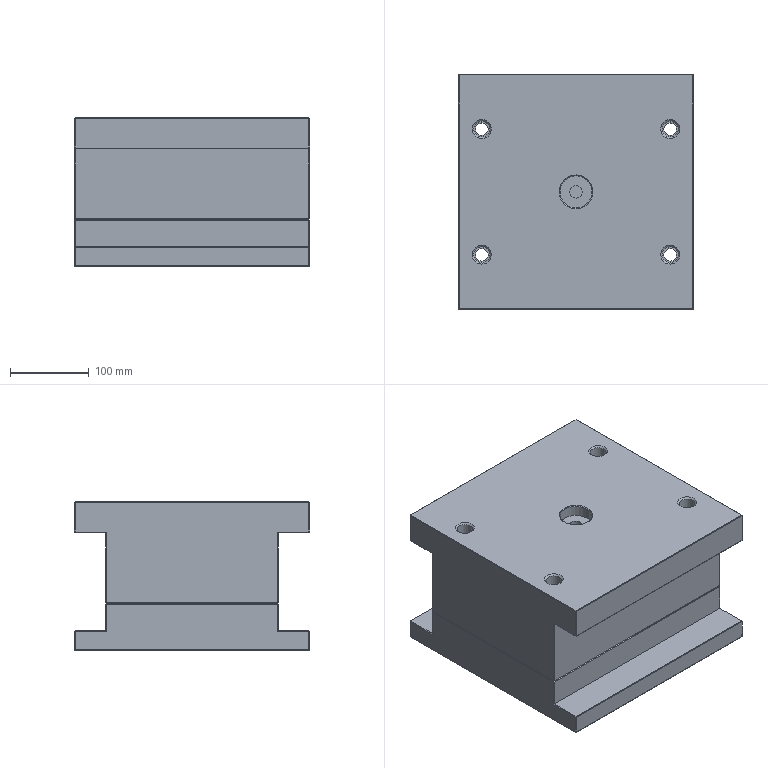NC program | NX | posted with a generic post | part box 300 x 300 x 190 mm
Lines 4668 to 6040 of 6235, first 962 of 1367 lines:
(HOLE_MILLING , TOOL : D10C)
N9334 T10 M6
N9336 G17 G43 G0 G90 X-120. Y80. Z30. S2000 H10 M3
N9338 Z0.5
N9340 G94 G3 X-118.55 Y78.55 R1.45 F1500.
N9342 X-117.1 Y80. R1.45
N9344 X-117.1 Y80. Z0.3 I-2.9 J0.
N9346 X-117.1 Y80. Z0.1 I-2.9 J0.
N9348 X-117.1 Y80. Z-0.1 I-2.9 J0.
N9350 X-117.1 Y80. Z-0.3 I-2.9 J0.
N9352 X-117.1 Y80. Z-0.5 I-2.9 J0.
N9354 X-117.1 Y80. Z-0.7 I-2.9 J0.
N9356 X-117.1 Y80. Z-0.9 I-2.9 J0.
N9358 X-117.1 Y80. Z-1.1 I-2.9 J0.
N9360 X-117.1 Y80. Z-1.3 I-2.9 J0.
N9362 X-117.1 Y80. Z-1.5 I-2.9 J0.
N9364 X-117.1 Y80. Z-1.7 I-2.9 J0.
N9366 X-117.1 Y80. Z-1.9 I-2.9 J0.
N9368 X-117.1 Y80. Z-2.1 I-2.9 J0.
N9370 X-117.1 Y80. Z-2.3 I-2.9 J0.
N9372 X-117.1 Y80. Z-2.5 I-2.9 J0.
N9374 X-117.1 Y80. Z-2.7 I-2.9 J0.
N9376 X-117.1 Y80. Z-2.9 I-2.9 J0.
N9378 X-117.1 Y80. Z-3.1 I-2.9 J0.
N9380 X-117.1 Y80. Z-3.3 I-2.9 J0.
N9382 X-117.1 Y80. Z-3.5 I-2.9 J0.
N9384 X-117.1 Y80. Z-3.7 I-2.9 J0.
N9386 X-117.1 Y80. Z-3.9 I-2.9 J0.
N9388 X-117.1 Y80. Z-4.1 I-2.9 J0.
N9390 X-117.1 Y80. Z-4.3 I-2.9 J0.
N9392 X-117.1 Y80. Z-4.5 I-2.9 J0.
N9394 X-117.1 Y80. Z-4.7 I-2.9 J0.
N9396 X-117.1 Y80. Z-4.9 I-2.9 J0.
N9398 X-117.1 Y80. Z-5.1 I-2.9 J0.
N9400 X-117.1 Y80. Z-5.3 I-2.9 J0.
N9402 X-117.1 Y80. Z-5.5 I-2.9 J0.
N9404 X-117.1 Y80. Z-5.7 I-2.9 J0.
N9406 X-117.1 Y80. Z-5.9 I-2.9 J0.
N9408 X-117.1 Y80. Z-6.1 I-2.9 J0.
N9410 X-117.1 Y80. Z-6.3 I-2.9 J0.
N9412 X-117.1 Y80. Z-6.5 I-2.9 J0.
N9414 X-117.1 Y80. Z-6.7 I-2.9 J0.
N9416 X-117.1 Y80. Z-6.9 I-2.9 J0.
N9418 X-117.1 Y80. Z-7.1 I-2.9 J0.
N9420 X-117.1 Y80. Z-7.3 I-2.9 J0.
N9422 X-117.1 Y80. Z-7.5 I-2.9 J0.
N9424 X-117.1 Y80. Z-7.7 I-2.9 J0.
N9426 X-117.1 Y80. Z-7.9 I-2.9 J0.
N9428 X-117.1 Y80. Z-8.1 I-2.9 J0.
N9430 X-117.1 Y80. Z-8.3 I-2.9 J0.
N9432 X-117.1 Y80. Z-8.5 I-2.9 J0.
N9434 X-117.1 Y80. Z-8.7 I-2.9 J0.
N9436 X-117.1 Y80. Z-8.9 I-2.9 J0.
N9438 X-117.1 Y80. Z-9.1 I-2.9 J0.
N9440 X-117.1 Y80. Z-9.3 I-2.9 J0.
N9442 X-117.1 Y80. Z-9.5 I-2.9 J0.
N9444 X-117.1 Y80. Z-9.7 I-2.9 J0.
N9446 X-117.1 Y80. Z-9.9 I-2.9 J0.
N9448 X-117.1 Y80. Z-10.1 I-2.9 J0.
N9450 X-117.1 Y80. Z-10.3 I-2.9 J0.
N9452 X-117.1 Y80. Z-10.5 I-2.9 J0.
N9454 X-117.1 Y80. Z-10.7 I-2.9 J0.
N9456 X-117.1 Y80. Z-10.9 I-2.9 J0.
N9458 X-117.1 Y80. Z-11.1 I-2.9 J0.
N9460 X-117.1 Y80. Z-11.3 I-2.9 J0.
N9462 X-117.1 Y80. Z-11.5 I-2.9 J0.
N9464 X-117.1 Y80. Z-11.7 I-2.9 J0.
N9466 X-117.1 Y80. Z-11.9 I-2.9 J0.
N9468 X-117.1 Y80. Z-12.1 I-2.9 J0.
N9470 X-117.1 Y80. Z-12.3 I-2.9 J0.
N9472 X-117.1 Y80. Z-12.5 I-2.9 J0.
N9474 X-117.1 Y80. Z-12.7 I-2.9 J0.
N9476 X-117.1 Y80. Z-12.9 I-2.9 J0.
N9478 X-117.1 Y80. Z-13.1 I-2.9 J0.
N9480 X-117.1 Y80. Z-13.3 I-2.9 J0.
N9482 X-117.1 Y80. Z-13.5 I-2.9 J0.
N9484 X-117.1 Y80. Z-13.7 I-2.9 J0.
N9486 X-117.1 Y80. Z-13.9 I-2.9 J0.
N9488 X-117.1 Y80. Z-14.1 I-2.9 J0.
N9490 X-117.1 Y80. Z-14.3 I-2.9 J0.
N9492 X-117.1 Y80. Z-14.5 I-2.9 J0.
N9494 X-117.1 Y80. Z-14.7 I-2.9 J0.
N9496 X-117.1 Y80. Z-14.9 I-2.9 J0.
N9498 X-117.1 Y80. Z-15.1 I-2.9 J0.
N9500 X-117.1 Y80. Z-15.3 I-2.9 J0.
N9502 X-117.1 Y80. Z-15.5 I-2.9 J0.
N9504 X-117.1 Y80. Z-15.7 I-2.9 J0.
N9506 X-117.1 Y80. Z-15.9 I-2.9 J0.
N9508 X-117.1 Y80. Z-16.1 I-2.9 J0.
N9510 X-117.1 Y80. Z-16.3 I-2.9 J0.
N9512 X-117.1 Y80. Z-16.5 I-2.9 J0.
N9514 X-117.1 Y80. Z-16.7 I-2.9 J0.
N9516 X-117.1 Y80. Z-16.9 I-2.9 J0.
N9518 X-117.1 Y80. Z-17.1 I-2.9 J0.
N9520 X-117.1 Y80. Z-17.3 I-2.9 J0.
N9522 X-117.1 Y80. Z-17.5 I-2.9 J0.
N9524 X-117.1 Y80. Z-17.7 I-2.9 J0.
N9526 X-117.1 Y80. Z-17.9 I-2.9 J0.
N9528 X-117.1 Y80. Z-18.1 I-2.9 J0.
N9530 X-117.1 Y80. Z-18.3 I-2.9 J0.
N9532 X-117.1 Y80. Z-18.5 I-2.9 J0.
N9534 X-117.1 Y80. Z-18.7 I-2.9 J0.
N9536 X-117.1 Y80. Z-18.9 I-2.9 J0.
N9538 X-117.1 Y80. Z-19.1 I-2.9 J0.
N9540 X-117.1 Y80. Z-19.3 I-2.9 J0.
N9542 X-117.1 Y80. Z-19.5 I-2.9 J0.
N9544 X-117.1 Y80. Z-19.7 I-2.9 J0.
N9546 X-117.1 Y80. Z-19.9 I-2.9 J0.
N9548 X-117.1 Y80. Z-20.1 I-2.9 J0.
N9550 X-117.1 Y80. Z-20.3 I-2.9 J0.
N9552 X-117.1 Y80. Z-20.5 I-2.9 J0.
N9554 X-117.1 Y80. Z-20.7 I-2.9 J0.
N9556 X-117.1 Y80. Z-20.9 I-2.9 J0.
N9558 X-117.1 Y80. Z-21.1 I-2.9 J0.
N9560 X-117.1 Y80. Z-21.3 I-2.9 J0.
N9562 X-117.1 Y80. Z-21.5 I-2.9 J0.
N9564 X-117.1 Y80. Z-21.7 I-2.9 J0.
N9566 X-117.1 Y80. Z-21.9 I-2.9 J0.
N9568 X-117.1 Y80. Z-22.1 I-2.9 J0.
N9570 X-117.1 Y80. Z-22.3 I-2.9 J0.
N9572 X-117.1 Y80. Z-22.5 I-2.9 J0.
N9574 X-117.1 Y80. Z-22.7 I-2.9 J0.
N9576 X-117.1 Y80. Z-22.9 I-2.9 J0.
N9578 X-117.1 Y80. Z-23.1 I-2.9 J0.
N9580 X-117.1 Y80. Z-23.3 I-2.9 J0.
N9582 X-117.1 Y80. Z-23.5 I-2.9 J0.
N9584 X-117.1 Y80. Z-23.7 I-2.9 J0.
N9586 X-117.1 Y80. Z-23.9 I-2.9 J0.
N9588 X-117.1 Y80. Z-24.1 I-2.9 J0.
N9590 X-117.1 Y80. Z-24.3 I-2.9 J0.
N9592 X-117.1 Y80. Z-24.5 I-2.9 J0.
N9594 X-117.1 Y80. Z-24.7 I-2.9 J0.
N9596 X-117.1 Y80. Z-24.9 I-2.9 J0.
N9598 X-117.1 Y80. Z-25.1 I-2.9 J0.
N9600 X-117.1 Y80. Z-25.3 I-2.9 J0.
N9602 X-117.1 Y80. Z-25.5 I-2.9 J0.
N9604 X-117.1 Y80. Z-25.7 I-2.9 J0.
N9606 X-117.1 Y80. Z-25.9 I-2.9 J0.
N9608 X-117.1 Y80. Z-26.1 I-2.9 J0.
N9610 X-117.1 Y80. Z-26.3 I-2.9 J0.
N9612 X-117.1 Y80. Z-26.5 I-2.9 J0.
N9614 X-117.1 Y80. Z-26.7 I-2.9 J0.
N9616 X-117.1 Y80. Z-26.9 I-2.9 J0.
N9618 X-117.1 Y80. Z-27.1 I-2.9 J0.
N9620 X-117.1 Y80. Z-27.3 I-2.9 J0.
N9622 X-117.1 Y80. Z-27.5 I-2.9 J0.
N9624 X-117.1 Y80. Z-27.7 I-2.9 J0.
N9626 X-117.1 Y80. Z-27.9 I-2.9 J0.
N9628 X-117.1 Y80. Z-28.1 I-2.9 J0.
N9630 X-117.1 Y80. Z-28.3 I-2.9 J0.
N9632 X-117.1 Y80. Z-28.5 I-2.9 J0.
N9634 X-117.1 Y80. Z-28.7 I-2.9 J0.
N9636 X-117.1 Y80. Z-28.9 I-2.9 J0.
N9638 X-117.1 Y80. Z-29.1 I-2.9 J0.
N9640 X-117.1 Y80. Z-29.3 I-2.9 J0.
N9642 X-117.1 Y80. Z-29.5 I-2.9 J0.
N9644 X-117.1 Y80. Z-29.7 I-2.9 J0.
N9646 X-117.1 Y80. Z-29.9 I-2.9 J0.
N9648 X-117.1 Y80. Z-30.1 I-2.9 J0.
N9650 X-117.1 Y80. Z-30.3 I-2.9 J0.
N9652 X-117.1 Y80. Z-30.5 I-2.9 J0.
N9654 X-117.1 Y80. Z-30.7 I-2.9 J0.
N9656 X-117.1 Y80. Z-30.9 I-2.9 J0.
N9658 X-117.1 Y80. Z-31.1 I-2.9 J0.
N9660 X-117.1 Y80. Z-31.3 I-2.9 J0.
N9662 X-117.1 Y80. Z-31.5 I-2.9 J0.
N9664 X-117.1 Y80. Z-31.7 I-2.9 J0.
N9666 X-117.1 Y80. Z-31.9 I-2.9 J0.
N9668 X-117.1 Y80. Z-32.1 I-2.9 J0.
N9670 X-117.1 Y80. Z-32.3 I-2.9 J0.
N9672 X-117.1 Y80. Z-32.5 I-2.9 J0.
N9674 X-117.1 Y80. Z-32.7 I-2.9 J0.
N9676 X-117.1 Y80. Z-32.9 I-2.9 J0.
N9678 X-117.1 Y80. Z-33.1 I-2.9 J0.
N9680 X-117.1 Y80. Z-33.3 I-2.9 J0.
N9682 X-117.1 Y80. Z-33.5 I-2.9 J0.
N9684 X-117.1 Y80. Z-33.7 I-2.9 J0.
N9686 X-117.1 Y80. Z-33.9 I-2.9 J0.
N9688 X-117.1 Y80. Z-34.1 I-2.9 J0.
N9690 X-117.1 Y80. Z-34.3 I-2.9 J0.
N9692 X-117.1 Y80. Z-34.5 I-2.9 J0.
N9694 X-117.1 Y80. Z-34.7 I-2.9 J0.
N9696 X-117.1 Y80. Z-34.9 I-2.9 J0.
N9698 X-117.1 Y80. Z-35.1 I-2.9 J0.
N9700 X-117.1 Y80. Z-35.3 I-2.9 J0.
N9702 X-117.1 Y80. Z-35.5 I-2.9 J0.
N9704 X-117.1 Y80. Z-35.7 I-2.9 J0.
N9706 X-117.1 Y80. Z-35.9 I-2.9 J0.
N9708 X-117.1 Y80. Z-36.1 I-2.9 J0.
N9710 X-117.1 Y80. Z-36.3 I-2.9 J0.
N9712 X-117.1 Y80. Z-36.5 I-2.9 J0.
N9714 X-117.1 Y80. Z-36.7 I-2.9 J0.
N9716 X-117.1 Y80. Z-36.9 I-2.9 J0.
N9718 X-117.1 Y80. Z-37.1 I-2.9 J0.
N9720 X-117.1 Y80. Z-37.3 I-2.9 J0.
N9722 X-117.1 Y80. Z-37.5 I-2.9 J0.
N9724 X-117.1 Y80. Z-37.7 I-2.9 J0.
N9726 X-117.1 Y80. Z-37.9 I-2.9 J0.
N9728 X-117.1 Y80. Z-38.1 I-2.9 J0.
N9730 X-117.1 Y80. Z-38.3 I-2.9 J0.
N9732 X-117.1 Y80. Z-38.5 I-2.9 J0.
N9734 X-117.1 Y80. Z-38.7 I-2.9 J0.
N9736 X-117.1 Y80. Z-38.9 I-2.9 J0.
N9738 X-117.1 Y80. Z-39.1 I-2.9 J0.
N9740 X-117.1 Y80. Z-39.3 I-2.9 J0.
N9742 X-117.1 Y80. Z-39.5 I-2.9 J0.
N9744 X-117.1 Y80. Z-39.7 I-2.9 J0.
N9746 X-117.1 Y80. Z-39.9 I-2.9 J0.
N9748 X-117.1 Y80. Z-40.1 I-2.9 J0.
N9750 X-117.1 Y80. Z-40.3 I-2.9 J0.
N9752 X-117.1 Y80. Z-40.5 I-2.9 J0.
N9754 X-117.1 Y80. Z-40.7 I-2.9 J0.
N9756 X-117.1 Y80. Z-40.9 I-2.9 J0.
N9758 X-117.1 Y80. Z-41.1 I-2.9 J0.
N9760 X-117.1 Y80. Z-41.3 I-2.9 J0.
N9762 X-117.1 Y80. Z-41.5 I-2.9 J0.
N9764 X-117.1 Y80. Z-41.7 I-2.9 J0.
N9766 X-117.1 Y80. Z-41.9 I-2.9 J0.
N9768 X-117.1 Y80. Z-42.1 I-2.9 J0.
N9770 X-117.1 Y80. Z-42.3 I-2.9 J0.
N9772 X-117.1 Y80. Z-42.5 I-2.9 J0.
N9774 X-117.1 Y80. Z-42.7 I-2.9 J0.
N9776 X-117.1 Y80. Z-42.9 I-2.9 J0.
N9778 X-117.1 Y80. Z-43.1 I-2.9 J0.
N9780 X-117.1 Y80. Z-43.3 I-2.9 J0.
N9782 X-117.1 Y80. Z-43.5 I-2.9 J0.
N9784 X-117.1 Y80. Z-43.7 I-2.9 J0.
N9786 X-117.1 Y80. Z-43.9 I-2.9 J0.
N9788 X-117.1 Y80. Z-44.1 I-2.9 J0.
N9790 X-117.1 Y80. Z-44.3 I-2.9 J0.
N9792 X-117.1 Y80. Z-44.5 I-2.9 J0.
N9794 X-117.1 Y80. Z-44.7 I-2.9 J0.
N9796 X-117.1 Y80. Z-44.9 I-2.9 J0.
N9798 X-117.1 Y80. Z-45.1 I-2.9 J0.
N9800 X-117.1 Y80. Z-45.3 I-2.9 J0.
N9802 X-117.1 Y80. Z-45.5 I-2.9 J0.
N9804 X-117.1 Y80. Z-45.7 I-2.9 J0.
N9806 X-117.1 Y80. Z-45.9 I-2.9 J0.
N9808 X-117.1 Y80. Z-46.1 I-2.9 J0.
N9810 X-117.1 Y80. Z-46.3 I-2.9 J0.
N9812 X-117.1 Y80. Z-46.5 I-2.9 J0.
N9814 X-117.1 Y80. Z-46.7 I-2.9 J0.
N9816 X-117.1 Y80. Z-46.9 I-2.9 J0.
N9818 X-117.1 Y80. Z-47.1 I-2.9 J0.
N9820 X-117.1 Y80. Z-47.3 I-2.9 J0.
N9822 X-117.1 Y80. Z-47.5 I-2.9 J0.
N9824 X-117.1 Y80. Z-47.7 I-2.9 J0.
N9826 X-117.1 Y80. Z-47.9 I-2.9 J0.
N9828 X-117.1 Y80. Z-48.1 I-2.9 J0.
N9830 X-117.1 Y80. Z-48.3 I-2.9 J0.
N9832 X-117.1 Y80. Z-48.5 I-2.9 J0.
N9834 X-117.1 Y80. Z-48.7 I-2.9 J0.
N9836 X-117.1 Y80. Z-48.9 I-2.9 J0.
N9838 X-117.1 Y80. Z-49.1 I-2.9 J0.
N9840 X-117.1 Y80. Z-49.3 I-2.9 J0.
N9842 X-117.1 Y80. Z-49.5 I-2.9 J0.
N9844 X-117.1 Y80. Z-49.7 I-2.9 J0.
N9846 X-117.1 Y80. Z-49.9 I-2.9 J0.
N9848 X-117.1 Y80. Z-50.1 I-2.9 J0.
N9850 X-117.1 Y80. Z-50.3 I-2.9 J0.
N9852 X-117.1 Y80. Z-50.5 I-2.9 J0.
N9854 X-117.1 Y80. Z-50.7 I-2.9 J0.
N9856 X-117.1 Y80. Z-50.9 I-2.9 J0.
N9858 X-117.1 Y80. Z-51.1 I-2.9 J0.
N9860 X-117.1 Y80. Z-51.3 I-2.9 J0.
N9862 X-117.1 Y80. Z-51.5 I-2.9 J0.
N9864 X-117.1 Y80. Z-51.7 I-2.9 J0.
N9866 X-117.1 Y80. Z-51.9 I-2.9 J0.
N9868 X-117.1 Y80. Z-52.1 I-2.9 J0.
N9870 X-117.1 Y80. Z-52.3 I-2.9 J0.
N9872 X-117.1 Y80. Z-52.5 I-2.9 J0.
N9874 X-117.1 Y80. Z-52.7 I-2.9 J0.
N9876 X-117.1 Y80. Z-52.9 I-2.9 J0.
N9878 X-117.1 Y80. Z-53.1 I-2.9 J0.
N9880 X-117.1 Y80. Z-53.3 I-2.9 J0.
N9882 X-117.1 Y80. Z-53.5 I-2.9 J0.
N9884 X-117.1 Y80. Z-53.7 I-2.9 J0.
N9886 X-117.1 Y80. Z-53.9 I-2.9 J0.
N9888 X-117.1 Y80. Z-54.1 I-2.9 J0.
N9890 X-117.1 Y80. Z-54.3 I-2.9 J0.
N9892 X-117.1 Y80. Z-54.5 I-2.9 J0.
N9894 X-117.1 Y80. Z-54.7 I-2.9 J0.
N9896 X-117.1 Y80. Z-54.9 I-2.9 J0.
N9898 X-117.1 Y80. Z-55.1 I-2.9 J0.
N9900 X-117.1 Y80. Z-55.3 I-2.9 J0.
N9902 X-117.1 Y80. Z-55.5 I-2.9 J0.
N9904 X-117.1 Y80. Z-55.7 I-2.9 J0.
N9906 X-117.1 Y80. Z-55.9 I-2.9 J0.
N9908 X-117.1 Y80. Z-56.1 I-2.9 J0.
N9910 X-117.1 Y80. Z-56.3 I-2.9 J0.
N9912 X-117.1 Y80. Z-56.5 I-2.9 J0.
N9914 X-117.1 Y80. Z-56.7 I-2.9 J0.
N9916 X-117.1 Y80. Z-56.9 I-2.9 J0.
N9918 X-117.1 Y80. Z-57.1 I-2.9 J0.
N9920 X-117.1 Y80. Z-57.3 I-2.9 J0.
N9922 X-117.1 Y80. Z-57.5 I-2.9 J0.
N9924 X-117.1 Y80. Z-57.7 I-2.9 J0.
N9926 X-117.1 Y80. Z-57.9 I-2.9 J0.
N9928 X-117.1 Y80. Z-58.1 I-2.9 J0.
N9930 X-117.1 Y80. Z-58.3 I-2.9 J0.
N9932 X-117.1 Y80. Z-58.5 I-2.9 J0.
N9934 X-117.1 Y80. Z-58.7 I-2.9 J0.
N9936 X-117.1 Y80. Z-58.9 I-2.9 J0.
N9938 X-117.1 Y80. Z-59.1 I-2.9 J0.
N9940 X-117.1 Y80. Z-59.3 I-2.9 J0.
N9942 X-117.1 Y80. Z-59.5 I-2.9 J0.
N9944 X-117.1 Y80. Z-59.7 I-2.9 J0.
N9946 X-117.1 Y80. Z-59.9 I-2.9 J0.
N9948 X-122.9 Y80. Z-60. I-2.9 J0.
N9950 X-120. Y77.1 R2.9
N9952 X-122.9 Y80. R-2.9
N9954 X-121.45 Y78.55 R1.45
N9956 X-120. Y80. R1.45
N9958 G0 Z30.
N9960 Y-80.
N9962 Z0.5
N9964 G3 X-118.55 Y-81.45 R1.45
N9966 X-117.1 Y-80. R1.45
N9968 X-117.1 Y-80. Z0.3 I-2.9 J0.
N9970 X-117.1 Y-80. Z0.1 I-2.9 J0.
N9972 X-117.1 Y-80. Z-0.1 I-2.9 J0.
N9974 X-117.1 Y-80. Z-0.3 I-2.9 J0.
N9976 X-117.1 Y-80. Z-0.5 I-2.9 J0.
N9978 X-117.1 Y-80. Z-0.7 I-2.9 J0.
N9980 X-117.1 Y-80. Z-0.9 I-2.9 J0.
N9982 X-117.1 Y-80. Z-1.1 I-2.9 J0.
N9984 X-117.1 Y-80. Z-1.3 I-2.9 J0.
N9986 X-117.1 Y-80. Z-1.5 I-2.9 J0.
N9988 X-117.1 Y-80. Z-1.7 I-2.9 J0.
N9990 X-117.1 Y-80. Z-1.9 I-2.9 J0.
N9992 X-117.1 Y-80. Z-2.1 I-2.9 J0.
N9994 X-117.1 Y-80. Z-2.3 I-2.9 J0.
N9996 X-117.1 Y-80. Z-2.5 I-2.9 J0.
N9998 X-117.1 Y-80. Z-2.7 I-2.9 J0.
N10000 X-117.1 Y-80. Z-2.9 I-2.9 J0.
N10002 X-117.1 Y-80. Z-3.1 I-2.9 J0.
N10004 X-117.1 Y-80. Z-3.3 I-2.9 J0.
N10006 X-117.1 Y-80. Z-3.5 I-2.9 J0.
N10008 X-117.1 Y-80. Z-3.7 I-2.9 J0.
N10010 X-117.1 Y-80. Z-3.9 I-2.9 J0.
N10012 X-117.1 Y-80. Z-4.1 I-2.9 J0.
N10014 X-117.1 Y-80. Z-4.3 I-2.9 J0.
N10016 X-117.1 Y-80. Z-4.5 I-2.9 J0.
N10018 X-117.1 Y-80. Z-4.7 I-2.9 J0.
N10020 X-117.1 Y-80. Z-4.9 I-2.9 J0.
N10022 X-117.1 Y-80. Z-5.1 I-2.9 J0.
N10024 X-117.1 Y-80. Z-5.3 I-2.9 J0.
N10026 X-117.1 Y-80. Z-5.5 I-2.9 J0.
N10028 X-117.1 Y-80. Z-5.7 I-2.9 J0.
N10030 X-117.1 Y-80. Z-5.9 I-2.9 J0.
N10032 X-117.1 Y-80. Z-6.1 I-2.9 J0.
N10034 X-117.1 Y-80. Z-6.3 I-2.9 J0.
N10036 X-117.1 Y-80. Z-6.5 I-2.9 J0.
N10038 X-117.1 Y-80. Z-6.7 I-2.9 J0.
N10040 X-117.1 Y-80. Z-6.9 I-2.9 J0.
N10042 X-117.1 Y-80. Z-7.1 I-2.9 J0.
N10044 X-117.1 Y-80. Z-7.3 I-2.9 J0.
N10046 X-117.1 Y-80. Z-7.5 I-2.9 J0.
N10048 X-117.1 Y-80. Z-7.7 I-2.9 J0.
N10050 X-117.1 Y-80. Z-7.9 I-2.9 J0.
N10052 X-117.1 Y-80. Z-8.1 I-2.9 J0.
N10054 X-117.1 Y-80. Z-8.3 I-2.9 J0.
N10056 X-117.1 Y-80. Z-8.5 I-2.9 J0.
N10058 X-117.1 Y-80. Z-8.7 I-2.9 J0.
N10060 X-117.1 Y-80. Z-8.9 I-2.9 J0.
N10062 X-117.1 Y-80. Z-9.1 I-2.9 J0.
N10064 X-117.1 Y-80. Z-9.3 I-2.9 J0.
N10066 X-117.1 Y-80. Z-9.5 I-2.9 J0.
N10068 X-117.1 Y-80. Z-9.7 I-2.9 J0.
N10070 X-117.1 Y-80. Z-9.9 I-2.9 J0.
N10072 X-117.1 Y-80. Z-10.1 I-2.9 J0.
N10074 X-117.1 Y-80. Z-10.3 I-2.9 J0.
N10076 X-117.1 Y-80. Z-10.5 I-2.9 J0.
N10078 X-117.1 Y-80. Z-10.7 I-2.9 J0.
N10080 X-117.1 Y-80. Z-10.9 I-2.9 J0.
N10082 X-117.1 Y-80. Z-11.1 I-2.9 J0.
N10084 X-117.1 Y-80. Z-11.3 I-2.9 J0.
N10086 X-117.1 Y-80. Z-11.5 I-2.9 J0.
N10088 X-117.1 Y-80. Z-11.7 I-2.9 J0.
N10090 X-117.1 Y-80. Z-11.9 I-2.9 J0.
N10092 X-117.1 Y-80. Z-12.1 I-2.9 J0.
N10094 X-117.1 Y-80. Z-12.3 I-2.9 J0.
N10096 X-117.1 Y-80. Z-12.5 I-2.9 J0.
N10098 X-117.1 Y-80. Z-12.7 I-2.9 J0.
N10100 X-117.1 Y-80. Z-12.9 I-2.9 J0.
N10102 X-117.1 Y-80. Z-13.1 I-2.9 J0.
N10104 X-117.1 Y-80. Z-13.3 I-2.9 J0.
N10106 X-117.1 Y-80. Z-13.5 I-2.9 J0.
N10108 X-117.1 Y-80. Z-13.7 I-2.9 J0.
N10110 X-117.1 Y-80. Z-13.9 I-2.9 J0.
N10112 X-117.1 Y-80. Z-14.1 I-2.9 J0.
N10114 X-117.1 Y-80. Z-14.3 I-2.9 J0.
N10116 X-117.1 Y-80. Z-14.5 I-2.9 J0.
N10118 X-117.1 Y-80. Z-14.7 I-2.9 J0.
N10120 X-117.1 Y-80. Z-14.9 I-2.9 J0.
N10122 X-117.1 Y-80. Z-15.1 I-2.9 J0.
N10124 X-117.1 Y-80. Z-15.3 I-2.9 J0.
N10126 X-117.1 Y-80. Z-15.5 I-2.9 J0.
N10128 X-117.1 Y-80. Z-15.7 I-2.9 J0.
N10130 X-117.1 Y-80. Z-15.9 I-2.9 J0.
N10132 X-117.1 Y-80. Z-16.1 I-2.9 J0.
N10134 X-117.1 Y-80. Z-16.3 I-2.9 J0.
N10136 X-117.1 Y-80. Z-16.5 I-2.9 J0.
N10138 X-117.1 Y-80. Z-16.7 I-2.9 J0.
N10140 X-117.1 Y-80. Z-16.9 I-2.9 J0.
N10142 X-117.1 Y-80. Z-17.1 I-2.9 J0.
N10144 X-117.1 Y-80. Z-17.3 I-2.9 J0.
N10146 X-117.1 Y-80. Z-17.5 I-2.9 J0.
N10148 X-117.1 Y-80. Z-17.7 I-2.9 J0.
N10150 X-117.1 Y-80. Z-17.9 I-2.9 J0.
N10152 X-117.1 Y-80. Z-18.1 I-2.9 J0.
N10154 X-117.1 Y-80. Z-18.3 I-2.9 J0.
N10156 X-117.1 Y-80. Z-18.5 I-2.9 J0.
N10158 X-117.1 Y-80. Z-18.7 I-2.9 J0.
N10160 X-117.1 Y-80. Z-18.9 I-2.9 J0.
N10162 X-117.1 Y-80. Z-19.1 I-2.9 J0.
N10164 X-117.1 Y-80. Z-19.3 I-2.9 J0.
N10166 X-117.1 Y-80. Z-19.5 I-2.9 J0.
N10168 X-117.1 Y-80. Z-19.7 I-2.9 J0.
N10170 X-117.1 Y-80. Z-19.9 I-2.9 J0.
N10172 X-117.1 Y-80. Z-20.1 I-2.9 J0.
N10174 X-117.1 Y-80. Z-20.3 I-2.9 J0.
N10176 X-117.1 Y-80. Z-20.5 I-2.9 J0.
N10178 X-117.1 Y-80. Z-20.7 I-2.9 J0.
N10180 X-117.1 Y-80. Z-20.9 I-2.9 J0.
N10182 X-117.1 Y-80. Z-21.1 I-2.9 J0.
N10184 X-117.1 Y-80. Z-21.3 I-2.9 J0.
N10186 X-117.1 Y-80. Z-21.5 I-2.9 J0.
N10188 X-117.1 Y-80. Z-21.7 I-2.9 J0.
N10190 X-117.1 Y-80. Z-21.9 I-2.9 J0.
N10192 X-117.1 Y-80. Z-22.1 I-2.9 J0.
N10194 X-117.1 Y-80. Z-22.3 I-2.9 J0.
N10196 X-117.1 Y-80. Z-22.5 I-2.9 J0.
N10198 X-117.1 Y-80. Z-22.7 I-2.9 J0.
N10200 X-117.1 Y-80. Z-22.9 I-2.9 J0.
N10202 X-117.1 Y-80. Z-23.1 I-2.9 J0.
N10204 X-117.1 Y-80. Z-23.3 I-2.9 J0.
N10206 X-117.1 Y-80. Z-23.5 I-2.9 J0.
N10208 X-117.1 Y-80. Z-23.7 I-2.9 J0.
N10210 X-117.1 Y-80. Z-23.9 I-2.9 J0.
N10212 X-117.1 Y-80. Z-24.1 I-2.9 J0.
N10214 X-117.1 Y-80. Z-24.3 I-2.9 J0.
N10216 X-117.1 Y-80. Z-24.5 I-2.9 J0.
N10218 X-117.1 Y-80. Z-24.7 I-2.9 J0.
N10220 X-117.1 Y-80. Z-24.9 I-2.9 J0.
N10222 X-117.1 Y-80. Z-25.1 I-2.9 J0.
N10224 X-117.1 Y-80. Z-25.3 I-2.9 J0.
N10226 X-117.1 Y-80. Z-25.5 I-2.9 J0.
N10228 X-117.1 Y-80. Z-25.7 I-2.9 J0.
N10230 X-117.1 Y-80. Z-25.9 I-2.9 J0.
N10232 X-117.1 Y-80. Z-26.1 I-2.9 J0.
N10234 X-117.1 Y-80. Z-26.3 I-2.9 J0.
N10236 X-117.1 Y-80. Z-26.5 I-2.9 J0.
N10238 X-117.1 Y-80. Z-26.7 I-2.9 J0.
N10240 X-117.1 Y-80. Z-26.9 I-2.9 J0.
N10242 X-117.1 Y-80. Z-27.1 I-2.9 J0.
N10244 X-117.1 Y-80. Z-27.3 I-2.9 J0.
N10246 X-117.1 Y-80. Z-27.5 I-2.9 J0.
N10248 X-117.1 Y-80. Z-27.7 I-2.9 J0.
N10250 X-117.1 Y-80. Z-27.9 I-2.9 J0.
N10252 X-117.1 Y-80. Z-28.1 I-2.9 J0.
N10254 X-117.1 Y-80. Z-28.3 I-2.9 J0.
N10256 X-117.1 Y-80. Z-28.5 I-2.9 J0.
N10258 X-117.1 Y-80. Z-28.7 I-2.9 J0.
N10260 X-117.1 Y-80. Z-28.9 I-2.9 J0.
N10262 X-117.1 Y-80. Z-29.1 I-2.9 J0.
N10264 X-117.1 Y-80. Z-29.3 I-2.9 J0.
N10266 X-117.1 Y-80. Z-29.5 I-2.9 J0.
N10268 X-117.1 Y-80. Z-29.7 I-2.9 J0.
N10270 X-117.1 Y-80. Z-29.9 I-2.9 J0.
N10272 X-117.1 Y-80. Z-30.1 I-2.9 J0.
N10274 X-117.1 Y-80. Z-30.3 I-2.9 J0.
N10276 X-117.1 Y-80. Z-30.5 I-2.9 J0.
N10278 X-117.1 Y-80. Z-30.7 I-2.9 J0.
N10280 X-117.1 Y-80. Z-30.9 I-2.9 J0.
N10282 X-117.1 Y-80. Z-31.1 I-2.9 J0.
N10284 X-117.1 Y-80. Z-31.3 I-2.9 J0.
N10286 X-117.1 Y-80. Z-31.5 I-2.9 J0.
N10288 X-117.1 Y-80. Z-31.7 I-2.9 J0.
N10290 X-117.1 Y-80. Z-31.9 I-2.9 J0.
N10292 X-117.1 Y-80. Z-32.1 I-2.9 J0.
N10294 X-117.1 Y-80. Z-32.3 I-2.9 J0.
N10296 X-117.1 Y-80. Z-32.5 I-2.9 J0.
N10298 X-117.1 Y-80. Z-32.7 I-2.9 J0.
N10300 X-117.1 Y-80. Z-32.9 I-2.9 J0.
N10302 X-117.1 Y-80. Z-33.1 I-2.9 J0.
N10304 X-117.1 Y-80. Z-33.3 I-2.9 J0.
N10306 X-117.1 Y-80. Z-33.5 I-2.9 J0.
N10308 X-117.1 Y-80. Z-33.7 I-2.9 J0.
N10310 X-117.1 Y-80. Z-33.9 I-2.9 J0.
N10312 X-117.1 Y-80. Z-34.1 I-2.9 J0.
N10314 X-117.1 Y-80. Z-34.3 I-2.9 J0.
N10316 X-117.1 Y-80. Z-34.5 I-2.9 J0.
N10318 X-117.1 Y-80. Z-34.7 I-2.9 J0.
N10320 X-117.1 Y-80. Z-34.9 I-2.9 J0.
N10322 X-117.1 Y-80. Z-35.1 I-2.9 J0.
N10324 X-117.1 Y-80. Z-35.3 I-2.9 J0.
N10326 X-117.1 Y-80. Z-35.5 I-2.9 J0.
N10328 X-117.1 Y-80. Z-35.7 I-2.9 J0.
N10330 X-117.1 Y-80. Z-35.9 I-2.9 J0.
N10332 X-117.1 Y-80. Z-36.1 I-2.9 J0.
N10334 X-117.1 Y-80. Z-36.3 I-2.9 J0.
N10336 X-117.1 Y-80. Z-36.5 I-2.9 J0.
N10338 X-117.1 Y-80. Z-36.7 I-2.9 J0.
N10340 X-117.1 Y-80. Z-36.9 I-2.9 J0.
N10342 X-117.1 Y-80. Z-37.1 I-2.9 J0.
N10344 X-117.1 Y-80. Z-37.3 I-2.9 J0.
N10346 X-117.1 Y-80. Z-37.5 I-2.9 J0.
N10348 X-117.1 Y-80. Z-37.7 I-2.9 J0.
N10350 X-117.1 Y-80. Z-37.9 I-2.9 J0.
N10352 X-117.1 Y-80. Z-38.1 I-2.9 J0.
N10354 X-117.1 Y-80. Z-38.3 I-2.9 J0.
N10356 X-117.1 Y-80. Z-38.5 I-2.9 J0.
N10358 X-117.1 Y-80. Z-38.7 I-2.9 J0.
N10360 X-117.1 Y-80. Z-38.9 I-2.9 J0.
N10362 X-117.1 Y-80. Z-39.1 I-2.9 J0.
N10364 X-117.1 Y-80. Z-39.3 I-2.9 J0.
N10366 X-117.1 Y-80. Z-39.5 I-2.9 J0.
N10368 X-117.1 Y-80. Z-39.7 I-2.9 J0.
N10370 X-117.1 Y-80. Z-39.9 I-2.9 J0.
N10372 X-117.1 Y-80. Z-40.1 I-2.9 J0.
N10374 X-117.1 Y-80. Z-40.3 I-2.9 J0.
N10376 X-117.1 Y-80. Z-40.5 I-2.9 J0.
N10378 X-117.1 Y-80. Z-40.7 I-2.9 J0.
N10380 X-117.1 Y-80. Z-40.9 I-2.9 J0.
N10382 X-117.1 Y-80. Z-41.1 I-2.9 J0.
N10384 X-117.1 Y-80. Z-41.3 I-2.9 J0.
N10386 X-117.1 Y-80. Z-41.5 I-2.9 J0.
N10388 X-117.1 Y-80. Z-41.7 I-2.9 J0.
N10390 X-117.1 Y-80. Z-41.9 I-2.9 J0.
N10392 X-117.1 Y-80. Z-42.1 I-2.9 J0.
N10394 X-117.1 Y-80. Z-42.3 I-2.9 J0.
N10396 X-117.1 Y-80. Z-42.5 I-2.9 J0.
N10398 X-117.1 Y-80. Z-42.7 I-2.9 J0.
N10400 X-117.1 Y-80. Z-42.9 I-2.9 J0.
N10402 X-117.1 Y-80. Z-43.1 I-2.9 J0.
N10404 X-117.1 Y-80. Z-43.3 I-2.9 J0.
N10406 X-117.1 Y-80. Z-43.5 I-2.9 J0.
N10408 X-117.1 Y-80. Z-43.7 I-2.9 J0.
N10410 X-117.1 Y-80. Z-43.9 I-2.9 J0.
N10412 X-117.1 Y-80. Z-44.1 I-2.9 J0.
N10414 X-117.1 Y-80. Z-44.3 I-2.9 J0.
N10416 X-117.1 Y-80. Z-44.5 I-2.9 J0.
N10418 X-117.1 Y-80. Z-44.7 I-2.9 J0.
N10420 X-117.1 Y-80. Z-44.9 I-2.9 J0.
N10422 X-117.1 Y-80. Z-45.1 I-2.9 J0.
N10424 X-117.1 Y-80. Z-45.3 I-2.9 J0.
N10426 X-117.1 Y-80. Z-45.5 I-2.9 J0.
N10428 X-117.1 Y-80. Z-45.7 I-2.9 J0.
N10430 X-117.1 Y-80. Z-45.9 I-2.9 J0.
N10432 X-117.1 Y-80. Z-46.1 I-2.9 J0.
N10434 X-117.1 Y-80. Z-46.3 I-2.9 J0.
N10436 X-117.1 Y-80. Z-46.5 I-2.9 J0.
N10438 X-117.1 Y-80. Z-46.7 I-2.9 J0.
N10440 X-117.1 Y-80. Z-46.9 I-2.9 J0.
N10442 X-117.1 Y-80. Z-47.1 I-2.9 J0.
N10444 X-117.1 Y-80. Z-47.3 I-2.9 J0.
N10446 X-117.1 Y-80. Z-47.5 I-2.9 J0.
N10448 X-117.1 Y-80. Z-47.7 I-2.9 J0.
N10450 X-117.1 Y-80. Z-47.9 I-2.9 J0.
N10452 X-117.1 Y-80. Z-48.1 I-2.9 J0.
N10454 X-117.1 Y-80. Z-48.3 I-2.9 J0.
N10456 X-117.1 Y-80. Z-48.5 I-2.9 J0.
N10458 X-117.1 Y-80. Z-48.7 I-2.9 J0.
N10460 X-117.1 Y-80. Z-48.9 I-2.9 J0.
N10462 X-117.1 Y-80. Z-49.1 I-2.9 J0.
N10464 X-117.1 Y-80. Z-49.3 I-2.9 J0.
N10466 X-117.1 Y-80. Z-49.5 I-2.9 J0.
N10468 X-117.1 Y-80. Z-49.7 I-2.9 J0.
N10470 X-117.1 Y-80. Z-49.9 I-2.9 J0.
N10472 X-117.1 Y-80. Z-50.1 I-2.9 J0.
N10474 X-117.1 Y-80. Z-50.3 I-2.9 J0.
N10476 X-117.1 Y-80. Z-50.5 I-2.9 J0.
N10478 X-117.1 Y-80. Z-50.7 I-2.9 J0.
N10480 X-117.1 Y-80. Z-50.9 I-2.9 J0.
N10482 X-117.1 Y-80. Z-51.1 I-2.9 J0.
N10484 X-117.1 Y-80. Z-51.3 I-2.9 J0.
N10486 X-117.1 Y-80. Z-51.5 I-2.9 J0.
N10488 X-117.1 Y-80. Z-51.7 I-2.9 J0.
N10490 X-117.1 Y-80. Z-51.9 I-2.9 J0.
N10492 X-117.1 Y-80. Z-52.1 I-2.9 J0.
N10494 X-117.1 Y-80. Z-52.3 I-2.9 J0.
N10496 X-117.1 Y-80. Z-52.5 I-2.9 J0.
N10498 X-117.1 Y-80. Z-52.7 I-2.9 J0.
N10500 X-117.1 Y-80. Z-52.9 I-2.9 J0.
N10502 X-117.1 Y-80. Z-53.1 I-2.9 J0.
N10504 X-117.1 Y-80. Z-53.3 I-2.9 J0.
N10506 X-117.1 Y-80. Z-53.5 I-2.9 J0.
N10508 X-117.1 Y-80. Z-53.7 I-2.9 J0.
N10510 X-117.1 Y-80. Z-53.9 I-2.9 J0.
N10512 X-117.1 Y-80. Z-54.1 I-2.9 J0.
N10514 X-117.1 Y-80. Z-54.3 I-2.9 J0.
N10516 X-117.1 Y-80. Z-54.5 I-2.9 J0.
N10518 X-117.1 Y-80. Z-54.7 I-2.9 J0.
N10520 X-117.1 Y-80. Z-54.9 I-2.9 J0.
N10522 X-117.1 Y-80. Z-55.1 I-2.9 J0.
N10524 X-117.1 Y-80. Z-55.3 I-2.9 J0.
N10526 X-117.1 Y-80. Z-55.5 I-2.9 J0.
N10528 X-117.1 Y-80. Z-55.7 I-2.9 J0.
N10530 X-117.1 Y-80. Z-55.9 I-2.9 J0.
N10532 X-117.1 Y-80. Z-56.1 I-2.9 J0.
N10534 X-117.1 Y-80. Z-56.3 I-2.9 J0.
N10536 X-117.1 Y-80. Z-56.5 I-2.9 J0.
N10538 X-117.1 Y-80. Z-56.7 I-2.9 J0.
N10540 X-117.1 Y-80. Z-56.9 I-2.9 J0.
N10542 X-117.1 Y-80. Z-57.1 I-2.9 J0.
N10544 X-117.1 Y-80. Z-57.3 I-2.9 J0.
N10546 X-117.1 Y-80. Z-57.5 I-2.9 J0.
N10548 X-117.1 Y-80. Z-57.7 I-2.9 J0.
N10550 X-117.1 Y-80. Z-57.9 I-2.9 J0.
N10552 X-117.1 Y-80. Z-58.1 I-2.9 J0.
N10554 X-117.1 Y-80. Z-58.3 I-2.9 J0.
N10556 X-117.1 Y-80. Z-58.5 I-2.9 J0.
N10558 X-117.1 Y-80. Z-58.7 I-2.9 J0.
N10560 X-117.1 Y-80. Z-58.9 I-2.9 J0.
N10562 X-117.1 Y-80. Z-59.1 I-2.9 J0.
N10564 X-117.1 Y-80. Z-59.3 I-2.9 J0.
N10566 X-117.1 Y-80. Z-59.5 I-2.9 J0.
N10568 X-117.1 Y-80. Z-59.7 I-2.9 J0.
N10570 X-117.1 Y-80. Z-59.9 I-2.9 J0.
N10572 X-122.9 Y-80. Z-60. I-2.9 J0.
N10574 X-120. Y-82.9 R2.9
N10576 X-122.9 Y-80. R-2.9
N10578 X-121.45 Y-81.45 R1.45
N10580 X-120. Y-80. R1.45
N10582 G0 Z30.
N10584 X120.
N10586 Z0.5
N10588 G3 X121.45 Y-81.45 R1.45
N10590 X122.9 Y-80. R1.45
N10592 X122.9 Y-80. Z0.3 I-2.9 J0.
N10594 X122.9 Y-80. Z0.1 I-2.9 J0.
N10596 X122.9 Y-80. Z-0.1 I-2.9 J0.
N10598 X122.9 Y-80. Z-0.3 I-2.9 J0.
N10600 X122.9 Y-80. Z-0.5 I-2.9 J0.
N10602 X122.9 Y-80. Z-0.7 I-2.9 J0.
N10604 X122.9 Y-80. Z-0.9 I-2.9 J0.
N10606 X122.9 Y-80. Z-1.1 I-2.9 J0.
N10608 X122.9 Y-80. Z-1.3 I-2.9 J0.
N10610 X122.9 Y-80. Z-1.5 I-2.9 J0.
N10612 X122.9 Y-80. Z-1.7 I-2.9 J0.
N10614 X122.9 Y-80. Z-1.9 I-2.9 J0.
N10616 X122.9 Y-80. Z-2.1 I-2.9 J0.
N10618 X122.9 Y-80. Z-2.3 I-2.9 J0.
N10620 X122.9 Y-80. Z-2.5 I-2.9 J0.
N10622 X122.9 Y-80. Z-2.7 I-2.9 J0.
N10624 X122.9 Y-80. Z-2.9 I-2.9 J0.
N10626 X122.9 Y-80. Z-3.1 I-2.9 J0.
N10628 X122.9 Y-80. Z-3.3 I-2.9 J0.
N10630 X122.9 Y-80. Z-3.5 I-2.9 J0.
N10632 X122.9 Y-80. Z-3.7 I-2.9 J0.
N10634 X122.9 Y-80. Z-3.9 I-2.9 J0.
N10636 X122.9 Y-80. Z-4.1 I-2.9 J0.
N10638 X122.9 Y-80. Z-4.3 I-2.9 J0.
N10640 X122.9 Y-80. Z-4.5 I-2.9 J0.
N10642 X122.9 Y-80. Z-4.7 I-2.9 J0.
N10644 X122.9 Y-80. Z-4.9 I-2.9 J0.
N10646 X122.9 Y-80. Z-5.1 I-2.9 J0.
N10648 X122.9 Y-80. Z-5.3 I-2.9 J0.
N10650 X122.9 Y-80. Z-5.5 I-2.9 J0.
N10652 X122.9 Y-80. Z-5.7 I-2.9 J0.
N10654 X122.9 Y-80. Z-5.9 I-2.9 J0.
N10656 X122.9 Y-80. Z-6.1 I-2.9 J0.
N10658 X122.9 Y-80. Z-6.3 I-2.9 J0.
N10660 X122.9 Y-80. Z-6.5 I-2.9 J0.
N10662 X122.9 Y-80. Z-6.7 I-2.9 J0.
N10664 X122.9 Y-80. Z-6.9 I-2.9 J0.
N10666 X122.9 Y-80. Z-7.1 I-2.9 J0.
N10668 X122.9 Y-80. Z-7.3 I-2.9 J0.
N10670 X122.9 Y-80. Z-7.5 I-2.9 J0.
N10672 X122.9 Y-80. Z-7.7 I-2.9 J0.
N10674 X122.9 Y-80. Z-7.9 I-2.9 J0.
N10676 X122.9 Y-80. Z-8.1 I-2.9 J0.
N10678 X122.9 Y-80. Z-8.3 I-2.9 J0.
N10680 X122.9 Y-80. Z-8.5 I-2.9 J0.
N10682 X122.9 Y-80. Z-8.7 I-2.9 J0.
N10684 X122.9 Y-80. Z-8.9 I-2.9 J0.
N10686 X122.9 Y-80. Z-9.1 I-2.9 J0.
N10688 X122.9 Y-80. Z-9.3 I-2.9 J0.
N10690 X122.9 Y-80. Z-9.5 I-2.9 J0.
N10692 X122.9 Y-80. Z-9.7 I-2.9 J0.
N10694 X122.9 Y-80. Z-9.9 I-2.9 J0.
N10696 X122.9 Y-80. Z-10.1 I-2.9 J0.
N10698 X122.9 Y-80. Z-10.3 I-2.9 J0.
N10700 X122.9 Y-80. Z-10.5 I-2.9 J0.
N10702 X122.9 Y-80. Z-10.7 I-2.9 J0.
N10704 X122.9 Y-80. Z-10.9 I-2.9 J0.
N10706 X122.9 Y-80. Z-11.1 I-2.9 J0.
N10708 X122.9 Y-80. Z-11.3 I-2.9 J0.
N10710 X122.9 Y-80. Z-11.5 I-2.9 J0.
N10712 X122.9 Y-80. Z-11.7 I-2.9 J0.
N10714 X122.9 Y-80. Z-11.9 I-2.9 J0.
N10716 X122.9 Y-80. Z-12.1 I-2.9 J0.
N10718 X122.9 Y-80. Z-12.3 I-2.9 J0.
N10720 X122.9 Y-80. Z-12.5 I-2.9 J0.
N10722 X122.9 Y-80. Z-12.7 I-2.9 J0.
N10724 X122.9 Y-80. Z-12.9 I-2.9 J0.
N10726 X122.9 Y-80. Z-13.1 I-2.9 J0.
N10728 X122.9 Y-80. Z-13.3 I-2.9 J0.
N10730 X122.9 Y-80. Z-13.5 I-2.9 J0.
N10732 X122.9 Y-80. Z-13.7 I-2.9 J0.
N10734 X122.9 Y-80. Z-13.9 I-2.9 J0.
N10736 X122.9 Y-80. Z-14.1 I-2.9 J0.
N10738 X122.9 Y-80. Z-14.3 I-2.9 J0.
N10740 X122.9 Y-80. Z-14.5 I-2.9 J0.
N10742 X122.9 Y-80. Z-14.7 I-2.9 J0.
N10744 X122.9 Y-80. Z-14.9 I-2.9 J0.
N10746 X122.9 Y-80. Z-15.1 I-2.9 J0.
N10748 X122.9 Y-80. Z-15.3 I-2.9 J0.
N10750 X122.9 Y-80. Z-15.5 I-2.9 J0.
N10752 X122.9 Y-80. Z-15.7 I-2.9 J0.
N10754 X122.9 Y-80. Z-15.9 I-2.9 J0.
N10756 X122.9 Y-80. Z-16.1 I-2.9 J0.
N10758 X122.9 Y-80. Z-16.3 I-2.9 J0.
N10760 X122.9 Y-80. Z-16.5 I-2.9 J0.
N10762 X122.9 Y-80. Z-16.7 I-2.9 J0.
N10764 X122.9 Y-80. Z-16.9 I-2.9 J0.
N10766 X122.9 Y-80. Z-17.1 I-2.9 J0.
N10768 X122.9 Y-80. Z-17.3 I-2.9 J0.
N10770 X122.9 Y-80. Z-17.5 I-2.9 J0.
N10772 X122.9 Y-80. Z-17.7 I-2.9 J0.
N10774 X122.9 Y-80. Z-17.9 I-2.9 J0.
N10776 X122.9 Y-80. Z-18.1 I-2.9 J0.
N10778 X122.9 Y-80. Z-18.3 I-2.9 J0.
N10780 X122.9 Y-80. Z-18.5 I-2.9 J0.
N10782 X122.9 Y-80. Z-18.7 I-2.9 J0.
N10784 X122.9 Y-80. Z-18.9 I-2.9 J0.
N10786 X122.9 Y-80. Z-19.1 I-2.9 J0.
N10788 X122.9 Y-80. Z-19.3 I-2.9 J0.
N10790 X122.9 Y-80. Z-19.5 I-2.9 J0.
N10792 X122.9 Y-80. Z-19.7 I-2.9 J0.
N10794 X122.9 Y-80. Z-19.9 I-2.9 J0.
N10796 X122.9 Y-80. Z-20.1 I-2.9 J0.
N10798 X122.9 Y-80. Z-20.3 I-2.9 J0.
N10800 X122.9 Y-80. Z-20.5 I-2.9 J0.
N10802 X122.9 Y-80. Z-20.7 I-2.9 J0.
N10804 X122.9 Y-80. Z-20.9 I-2.9 J0.
N10806 X122.9 Y-80. Z-21.1 I-2.9 J0.
N10808 X122.9 Y-80. Z-21.3 I-2.9 J0.
N10810 X122.9 Y-80. Z-21.5 I-2.9 J0.
N10812 X122.9 Y-80. Z-21.7 I-2.9 J0.
N10814 X122.9 Y-80. Z-21.9 I-2.9 J0.
N10816 X122.9 Y-80. Z-22.1 I-2.9 J0.
N10818 X122.9 Y-80. Z-22.3 I-2.9 J0.
N10820 X122.9 Y-80. Z-22.5 I-2.9 J0.
N10822 X122.9 Y-80. Z-22.7 I-2.9 J0.
N10824 X122.9 Y-80. Z-22.9 I-2.9 J0.
N10826 X122.9 Y-80. Z-23.1 I-2.9 J0.
N10828 X122.9 Y-80. Z-23.3 I-2.9 J0.
N10830 X122.9 Y-80. Z-23.5 I-2.9 J0.
N10832 X122.9 Y-80. Z-23.7 I-2.9 J0.
N10834 X122.9 Y-80. Z-23.9 I-2.9 J0.
N10836 X122.9 Y-80. Z-24.1 I-2.9 J0.
N10838 X122.9 Y-80. Z-24.3 I-2.9 J0.
N10840 X122.9 Y-80. Z-24.5 I-2.9 J0.
N10842 X122.9 Y-80. Z-24.7 I-2.9 J0.
N10844 X122.9 Y-80. Z-24.9 I-2.9 J0.
N10846 X122.9 Y-80. Z-25.1 I-2.9 J0.
N10848 X122.9 Y-80. Z-25.3 I-2.9 J0.
N10850 X122.9 Y-80. Z-25.5 I-2.9 J0.
N10852 X122.9 Y-80. Z-25.7 I-2.9 J0.
N10854 X122.9 Y-80. Z-25.9 I-2.9 J0.
N10856 X122.9 Y-80. Z-26.1 I-2.9 J0.
N10858 X122.9 Y-80. Z-26.3 I-2.9 J0.
N10860 X122.9 Y-80. Z-26.5 I-2.9 J0.
N10862 X122.9 Y-80. Z-26.7 I-2.9 J0.
N10864 X122.9 Y-80. Z-26.9 I-2.9 J0.
N10866 X122.9 Y-80. Z-27.1 I-2.9 J0.
N10868 X122.9 Y-80. Z-27.3 I-2.9 J0.
N10870 X122.9 Y-80. Z-27.5 I-2.9 J0.
N10872 X122.9 Y-80. Z-27.7 I-2.9 J0.
N10874 X122.9 Y-80. Z-27.9 I-2.9 J0.
N10876 X122.9 Y-80. Z-28.1 I-2.9 J0.
N10878 X122.9 Y-80. Z-28.3 I-2.9 J0.
N10880 X122.9 Y-80. Z-28.5 I-2.9 J0.
N10882 X122.9 Y-80. Z-28.7 I-2.9 J0.
N10884 X122.9 Y-80. Z-28.9 I-2.9 J0.
N10886 X122.9 Y-80. Z-29.1 I-2.9 J0.
N10888 X122.9 Y-80. Z-29.3 I-2.9 J0.
N10890 X122.9 Y-80. Z-29.5 I-2.9 J0.
N10892 X122.9 Y-80. Z-29.7 I-2.9 J0.
N10894 X122.9 Y-80. Z-29.9 I-2.9 J0.
N10896 X122.9 Y-80. Z-30.1 I-2.9 J0.
N10898 X122.9 Y-80. Z-30.3 I-2.9 J0.
N10900 X122.9 Y-80. Z-30.5 I-2.9 J0.
N10902 X122.9 Y-80. Z-30.7 I-2.9 J0.
N10904 X122.9 Y-80. Z-30.9 I-2.9 J0.
N10906 X122.9 Y-80. Z-31.1 I-2.9 J0.
N10908 X122.9 Y-80. Z-31.3 I-2.9 J0.
N10910 X122.9 Y-80. Z-31.5 I-2.9 J0.
N10912 X122.9 Y-80. Z-31.7 I-2.9 J0.
N10914 X122.9 Y-80. Z-31.9 I-2.9 J0.
N10916 X122.9 Y-80. Z-32.1 I-2.9 J0.
N10918 X122.9 Y-80. Z-32.3 I-2.9 J0.
N10920 X122.9 Y-80. Z-32.5 I-2.9 J0.
N10922 X122.9 Y-80. Z-32.7 I-2.9 J0.
N10924 X122.9 Y-80. Z-32.9 I-2.9 J0.
N10926 X122.9 Y-80. Z-33.1 I-2.9 J0.
N10928 X122.9 Y-80. Z-33.3 I-2.9 J0.
N10930 X122.9 Y-80. Z-33.5 I-2.9 J0.
N10932 X122.9 Y-80. Z-33.7 I-2.9 J0.
N10934 X122.9 Y-80. Z-33.9 I-2.9 J0.
N10936 X122.9 Y-80. Z-34.1 I-2.9 J0.
N10938 X122.9 Y-80. Z-34.3 I-2.9 J0.
N10940 X122.9 Y-80. Z-34.5 I-2.9 J0.
N10942 X122.9 Y-80. Z-34.7 I-2.9 J0.
N10944 X122.9 Y-80. Z-34.9 I-2.9 J0.
N10946 X122.9 Y-80. Z-35.1 I-2.9 J0.
N10948 X122.9 Y-80. Z-35.3 I-2.9 J0.
N10950 X122.9 Y-80. Z-35.5 I-2.9 J0.
N10952 X122.9 Y-80. Z-35.7 I-2.9 J0.
N10954 X122.9 Y-80. Z-35.9 I-2.9 J0.
N10956 X122.9 Y-80. Z-36.1 I-2.9 J0.
N10958 X122.9 Y-80. Z-36.3 I-2.9 J0.
N10960 X122.9 Y-80. Z-36.5 I-2.9 J0.
N10962 X122.9 Y-80. Z-36.7 I-2.9 J0.
N10964 X122.9 Y-80. Z-36.9 I-2.9 J0.
N10966 X122.9 Y-80. Z-37.1 I-2.9 J0.
N10968 X122.9 Y-80. Z-37.3 I-2.9 J0.
N10970 X122.9 Y-80. Z-37.5 I-2.9 J0.
N10972 X122.9 Y-80. Z-37.7 I-2.9 J0.
N10974 X122.9 Y-80. Z-37.9 I-2.9 J0.
N10976 X122.9 Y-80. Z-38.1 I-2.9 J0.
N10978 X122.9 Y-80. Z-38.3 I-2.9 J0.
N10980 X122.9 Y-80. Z-38.5 I-2.9 J0.
N10982 X122.9 Y-80. Z-38.7 I-2.9 J0.
N10984 X122.9 Y-80. Z-38.9 I-2.9 J0.
N10986 X122.9 Y-80. Z-39.1 I-2.9 J0.
N10988 X122.9 Y-80. Z-39.3 I-2.9 J0.
N10990 X122.9 Y-80. Z-39.5 I-2.9 J0.
N10992 X122.9 Y-80. Z-39.7 I-2.9 J0.
N10994 X122.9 Y-80. Z-39.9 I-2.9 J0.
N10996 X122.9 Y-80. Z-40.1 I-2.9 J0.
N10998 X122.9 Y-80. Z-40.3 I-2.9 J0.
N11000 X122.9 Y-80. Z-40.5 I-2.9 J0.
N11002 X122.9 Y-80. Z-40.7 I-2.9 J0.
N11004 X122.9 Y-80. Z-40.9 I-2.9 J0.
N11006 X122.9 Y-80. Z-41.1 I-2.9 J0.
N11008 X122.9 Y-80. Z-41.3 I-2.9 J0.
N11010 X122.9 Y-80. Z-41.5 I-2.9 J0.
N11012 X122.9 Y-80. Z-41.7 I-2.9 J0.
N11014 X122.9 Y-80. Z-41.9 I-2.9 J0.
N11016 X122.9 Y-80. Z-42.1 I-2.9 J0.
N11018 X122.9 Y-80. Z-42.3 I-2.9 J0.
N11020 X122.9 Y-80. Z-42.5 I-2.9 J0.
N11022 X122.9 Y-80. Z-42.7 I-2.9 J0.
N11024 X122.9 Y-80. Z-42.9 I-2.9 J0.
N11026 X122.9 Y-80. Z-43.1 I-2.9 J0.
N11028 X122.9 Y-80. Z-43.3 I-2.9 J0.
N11030 X122.9 Y-80. Z-43.5 I-2.9 J0.
N11032 X122.9 Y-80. Z-43.7 I-2.9 J0.
N11034 X122.9 Y-80. Z-43.9 I-2.9 J0.
N11036 X122.9 Y-80. Z-44.1 I-2.9 J0.
N11038 X122.9 Y-80. Z-44.3 I-2.9 J0.
N11040 X122.9 Y-80. Z-44.5 I-2.9 J0.
N11042 X122.9 Y-80. Z-44.7 I-2.9 J0.
N11044 X122.9 Y-80. Z-44.9 I-2.9 J0.
N11046 X122.9 Y-80. Z-45.1 I-2.9 J0.
N11048 X122.9 Y-80. Z-45.3 I-2.9 J0.
N11050 X122.9 Y-80. Z-45.5 I-2.9 J0.
N11052 X122.9 Y-80. Z-45.7 I-2.9 J0.
N11054 X122.9 Y-80. Z-45.9 I-2.9 J0.
N11056 X122.9 Y-80. Z-46.1 I-2.9 J0.
N11058 X122.9 Y-80. Z-46.3 I-2.9 J0.
N11060 X122.9 Y-80. Z-46.5 I-2.9 J0.
N11062 X122.9 Y-80. Z-46.7 I-2.9 J0.
N11064 X122.9 Y-80. Z-46.9 I-2.9 J0.
N11066 X122.9 Y-80. Z-47.1 I-2.9 J0.
N11068 X122.9 Y-80. Z-47.3 I-2.9 J0.
N11070 X122.9 Y-80. Z-47.5 I-2.9 J0.
N11072 X122.9 Y-80. Z-47.7 I-2.9 J0.
N11074 X122.9 Y-80. Z-47.9 I-2.9 J0.
N11076 X122.9 Y-80. Z-48.1 I-2.9 J0.
N11078 X122.9 Y-80. Z-48.3 I-2.9 J0.
N11080 X122.9 Y-80. Z-48.5 I-2.9 J0.
N11082 X122.9 Y-80. Z-48.7 I-2.9 J0.
N11084 X122.9 Y-80. Z-48.9 I-2.9 J0.
N11086 X122.9 Y-80. Z-49.1 I-2.9 J0.
N11088 X122.9 Y-80. Z-49.3 I-2.9 J0.
N11090 X122.9 Y-80. Z-49.5 I-2.9 J0.
N11092 X122.9 Y-80. Z-49.7 I-2.9 J0.
N11094 X122.9 Y-80. Z-49.9 I-2.9 J0.
N11096 X122.9 Y-80. Z-50.1 I-2.9 J0.
N11098 X122.9 Y-80. Z-50.3 I-2.9 J0.
N11100 X122.9 Y-80. Z-50.5 I-2.9 J0.
N11102 X122.9 Y-80. Z-50.7 I-2.9 J0.
N11104 X122.9 Y-80. Z-50.9 I-2.9 J0.
N11106 X122.9 Y-80. Z-51.1 I-2.9 J0.
N11108 X122.9 Y-80. Z-51.3 I-2.9 J0.
N11110 X122.9 Y-80. Z-51.5 I-2.9 J0.
N11112 X122.9 Y-80. Z-51.7 I-2.9 J0.
N11114 X122.9 Y-80. Z-51.9 I-2.9 J0.
N11116 X122.9 Y-80. Z-52.1 I-2.9 J0.
N11118 X122.9 Y-80. Z-52.3 I-2.9 J0.
N11120 X122.9 Y-80. Z-52.5 I-2.9 J0.
N11122 X122.9 Y-80. Z-52.7 I-2.9 J0.
N11124 X122.9 Y-80. Z-52.9 I-2.9 J0.
N11126 X122.9 Y-80. Z-53.1 I-2.9 J0.
N11128 X122.9 Y-80. Z-53.3 I-2.9 J0.
N11130 X122.9 Y-80. Z-53.5 I-2.9 J0.
N11132 X122.9 Y-80. Z-53.7 I-2.9 J0.
N11134 X122.9 Y-80. Z-53.9 I-2.9 J0.
N11136 X122.9 Y-80. Z-54.1 I-2.9 J0.
N11138 X122.9 Y-80. Z-54.3 I-2.9 J0.
N11140 X122.9 Y-80. Z-54.5 I-2.9 J0.
N11142 X122.9 Y-80. Z-54.7 I-2.9 J0.
N11144 X122.9 Y-80. Z-54.9 I-2.9 J0.
N11146 X122.9 Y-80. Z-55.1 I-2.9 J0.
N11148 X122.9 Y-80. Z-55.3 I-2.9 J0.
N11150 X122.9 Y-80. Z-55.5 I-2.9 J0.
N11152 X122.9 Y-80. Z-55.7 I-2.9 J0.
N11154 X122.9 Y-80. Z-55.9 I-2.9 J0.
N11156 X122.9 Y-80. Z-56.1 I-2.9 J0.
N11158 X122.9 Y-80. Z-56.3 I-2.9 J0.
N11160 X122.9 Y-80. Z-56.5 I-2.9 J0.
N11162 X122.9 Y-80. Z-56.7 I-2.9 J0.
N11164 X122.9 Y-80. Z-56.9 I-2.9 J0.
N11166 X122.9 Y-80. Z-57.1 I-2.9 J0.
N11168 X122.9 Y-80. Z-57.3 I-2.9 J0.
N11170 X122.9 Y-80. Z-57.5 I-2.9 J0.
N11172 X122.9 Y-80. Z-57.7 I-2.9 J0.
N11174 X122.9 Y-80. Z-57.9 I-2.9 J0.
N11176 X122.9 Y-80. Z-58.1 I-2.9 J0.
N11178 X122.9 Y-80. Z-58.3 I-2.9 J0.
N11180 X122.9 Y-80. Z-58.5 I-2.9 J0.
N11182 X122.9 Y-80. Z-58.7 I-2.9 J0.
N11184 X122.9 Y-80. Z-58.9 I-2.9 J0.
N11186 X122.9 Y-80. Z-59.1 I-2.9 J0.
N11188 X122.9 Y-80. Z-59.3 I-2.9 J0.
N11190 X122.9 Y-80. Z-59.5 I-2.9 J0.
N11192 X122.9 Y-80. Z-59.7 I-2.9 J0.
N11194 X122.9 Y-80. Z-59.9 I-2.9 J0.
N11196 X117.1 Y-80. Z-60. I-2.9 J0.
N11198 X120. Y-82.9 R2.9
N11200 X117.1 Y-80. R-2.9
N11202 X118.55 Y-81.45 R1.45
N11204 X120. Y-80. R1.45
N11206 G0 Z30.
N11208 Y80.
N11210 Z0.5
N11212 G3 X121.45 Y78.55 R1.45
N11214 X122.9 Y80. R1.45
N11216 X122.9 Y80. Z0.3 I-2.9 J0.
N11218 X122.9 Y80. Z0.1 I-2.9 J0.
N11220 X122.9 Y80. Z-0.1 I-2.9 J0.
N11222 X122.9 Y80. Z-0.3 I-2.9 J0.
N11224 X122.9 Y80. Z-0.5 I-2.9 J0.
N11226 X122.9 Y80. Z-0.7 I-2.9 J0.
N11228 X122.9 Y80. Z-0.9 I-2.9 J0.
N11230 X122.9 Y80. Z-1.1 I-2.9 J0.
N11232 X122.9 Y80. Z-1.3 I-2.9 J0.
N11234 X122.9 Y80. Z-1.5 I-2.9 J0.
N11236 X122.9 Y80. Z-1.7 I-2.9 J0.
N11238 X122.9 Y80. Z-1.9 I-2.9 J0.
N11240 X122.9 Y80. Z-2.1 I-2.9 J0.
N11242 X122.9 Y80. Z-2.3 I-2.9 J0.
N11244 X122.9 Y80. Z-2.5 I-2.9 J0.
N11246 X122.9 Y80. Z-2.7 I-2.9 J0.
N11248 X122.9 Y80. Z-2.9 I-2.9 J0.
N11250 X122.9 Y80. Z-3.1 I-2.9 J0.
N11252 X122.9 Y80. Z-3.3 I-2.9 J0.
N11254 X122.9 Y80. Z-3.5 I-2.9 J0.